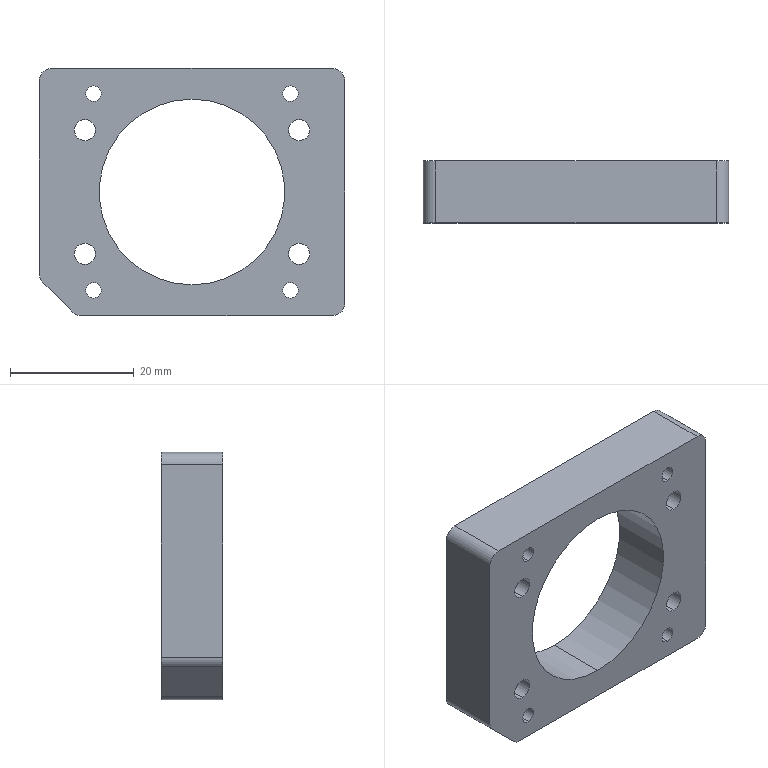Part | STEP file | 06-05KK60伺服连接Plate(KK60 Upper银伺服连接Plate) | 1 solid | 42 faces | box 49.4 x 10 x 40 mm | volume 11250 mm3 | cylinder 31 | plane 11 | commonest cylinder face diameters 2.5 x8 3.4 x8 6.5 x8 4 x5 30 x2
STEP:
#1=CARTESIAN_POINT('',(15.91,0.,14.66));
#2=VERTEX_POINT('',#1);
#3=CARTESIAN_POINT('',(15.91,0.,17.16));
#4=VERTEX_POINT('',#3);
#5=CARTESIAN_POINT('',(15.91,0.,15.91));
#6=DIRECTION('',(0.,1.,0.));
#7=DIRECTION('',(0.,0.,1.));
#8=AXIS2_PLACEMENT_3D('',#5,#6,#7);
#9=CIRCLE('',#8,1.25);
#10=EDGE_CURVE('',#2,#4,#9,.T.);
#11=ORIENTED_EDGE('',*,*,#10,.F.);
#12=CARTESIAN_POINT('',(15.91,10.,14.66));
#13=VERTEX_POINT('',#12);
#14=CARTESIAN_POINT('',(15.91,10.,14.66));
#15=DIRECTION('',(0.,1.,0.));
#16=VECTOR('',#15,1000.);
#17=LINE('',#14,#16);
#18=EDGE_CURVE('',#2,#13,#17,.T.);
#19=ORIENTED_EDGE('',*,*,#18,.T.);
#20=CARTESIAN_POINT('',(15.91,10.,17.16));
#21=VERTEX_POINT('',#20);
#22=CARTESIAN_POINT('',(15.91,10.,15.91));
#23=DIRECTION('',(0.,1.,0.));
#24=DIRECTION('',(0.,0.,1.));
#25=AXIS2_PLACEMENT_3D('',#22,#23,#24);
#26=CIRCLE('',#25,1.25);
#27=EDGE_CURVE('',#13,#21,#26,.T.);
#28=ORIENTED_EDGE('',*,*,#27,.T.);
#29=CARTESIAN_POINT('',(15.91,10.,17.16));
#30=DIRECTION('',(0.,1.,0.));
#31=VECTOR('',#30,1000.);
#32=LINE('',#29,#31);
#33=EDGE_CURVE('',#4,#21,#32,.T.);
#34=ORIENTED_EDGE('',*,*,#33,.F.);
#35=EDGE_LOOP('',(#11,#19,#28,#34));
#36=FACE_OUTER_BOUND('',#35,.T.);
#37=CARTESIAN_POINT('',(15.91,10.,15.91));
#38=DIRECTION('',(0.,1.,0.));
#39=DIRECTION('',(0.,0.,1.));
#40=AXIS2_PLACEMENT_3D('',#37,#38,#39);
#41=CYLINDRICAL_SURFACE('',#40,1.25);
#42=ADVANCED_FACE('',(#36),#41,.F.);
#43=CARTESIAN_POINT('',(-15.91,0.,14.66));
#44=VERTEX_POINT('',#43);
#45=CARTESIAN_POINT('',(-15.91,0.,17.16));
#46=VERTEX_POINT('',#45);
#47=CARTESIAN_POINT('',(-15.91,0.,15.91));
#48=DIRECTION('',(0.,1.,0.));
#49=DIRECTION('',(0.,0.,1.));
#50=AXIS2_PLACEMENT_3D('',#47,#48,#49);
#51=CIRCLE('',#50,1.25);
#52=EDGE_CURVE('',#44,#46,#51,.T.);
#53=ORIENTED_EDGE('',*,*,#52,.F.);
#54=CARTESIAN_POINT('',(-15.91,10.,14.66));
#55=VERTEX_POINT('',#54);
#56=CARTESIAN_POINT('',(-15.91,10.,14.66));
#57=DIRECTION('',(0.,1.,0.));
#58=VECTOR('',#57,1000.);
#59=LINE('',#56,#58);
#60=EDGE_CURVE('',#44,#55,#59,.T.);
#61=ORIENTED_EDGE('',*,*,#60,.T.);
#62=CARTESIAN_POINT('',(-15.91,10.,17.16));
#63=VERTEX_POINT('',#62);
#64=CARTESIAN_POINT('',(-15.91,10.,15.91));
#65=DIRECTION('',(0.,1.,0.));
#66=DIRECTION('',(0.,0.,1.));
#67=AXIS2_PLACEMENT_3D('',#64,#65,#66);
#68=CIRCLE('',#67,1.25);
#69=EDGE_CURVE('',#55,#63,#68,.T.);
#70=ORIENTED_EDGE('',*,*,#69,.T.);
#71=CARTESIAN_POINT('',(-15.91,10.,17.16));
#72=DIRECTION('',(0.,1.,0.));
#73=VECTOR('',#72,1000.);
#74=LINE('',#71,#73);
#75=EDGE_CURVE('',#46,#63,#74,.T.);
#76=ORIENTED_EDGE('',*,*,#75,.F.);
#77=EDGE_LOOP('',(#53,#61,#70,#76));
#78=FACE_OUTER_BOUND('',#77,.T.);
#79=CARTESIAN_POINT('',(-15.91,10.,15.91));
#80=DIRECTION('',(0.,1.,0.));
#81=DIRECTION('',(0.,0.,1.));
#82=AXIS2_PLACEMENT_3D('',#79,#80,#81);
#83=CYLINDRICAL_SURFACE('',#82,1.25);
#84=ADVANCED_FACE('',(#78),#83,.F.);
#85=CARTESIAN_POINT('',(-15.91,0.,-17.16));
#86=VERTEX_POINT('',#85);
#87=CARTESIAN_POINT('',(-15.91,0.,-14.66));
#88=VERTEX_POINT('',#87);
#89=CARTESIAN_POINT('',(-15.91,0.,-15.91));
#90=DIRECTION('',(0.,1.,0.));
#91=DIRECTION('',(0.,0.,1.));
#92=AXIS2_PLACEMENT_3D('',#89,#90,#91);
#93=CIRCLE('',#92,1.25);
#94=EDGE_CURVE('',#86,#88,#93,.T.);
#95=ORIENTED_EDGE('',*,*,#94,.F.);
#96=CARTESIAN_POINT('',(-15.91,10.,-17.16));
#97=VERTEX_POINT('',#96);
#98=CARTESIAN_POINT('',(-15.91,10.,-17.16));
#99=DIRECTION('',(0.,1.,0.));
#100=VECTOR('',#99,1000.);
#101=LINE('',#98,#100);
#102=EDGE_CURVE('',#86,#97,#101,.T.);
#103=ORIENTED_EDGE('',*,*,#102,.T.);
#104=CARTESIAN_POINT('',(-15.91,10.,-14.66));
#105=VERTEX_POINT('',#104);
#106=CARTESIAN_POINT('',(-15.91,10.,-15.91));
#107=DIRECTION('',(0.,1.,0.));
#108=DIRECTION('',(0.,0.,1.));
#109=AXIS2_PLACEMENT_3D('',#106,#107,#108);
#110=CIRCLE('',#109,1.25);
#111=EDGE_CURVE('',#97,#105,#110,.T.);
#112=ORIENTED_EDGE('',*,*,#111,.T.);
#113=CARTESIAN_POINT('',(-15.91,10.,-14.66));
#114=DIRECTION('',(0.,1.,0.));
#115=VECTOR('',#114,1000.);
#116=LINE('',#113,#115);
#117=EDGE_CURVE('',#88,#105,#116,.T.);
#118=ORIENTED_EDGE('',*,*,#117,.F.);
#119=EDGE_LOOP('',(#95,#103,#112,#118));
#120=FACE_OUTER_BOUND('',#119,.T.);
#121=CARTESIAN_POINT('',(-15.91,10.,-15.91));
#122=DIRECTION('',(0.,1.,0.));
#123=DIRECTION('',(0.,0.,1.));
#124=AXIS2_PLACEMENT_3D('',#121,#122,#123);
#125=CYLINDRICAL_SURFACE('',#124,1.25);
#126=ADVANCED_FACE('',(#120),#125,.F.);
#127=CARTESIAN_POINT('',(15.91,0.,-17.16));
#128=VERTEX_POINT('',#127);
#129=CARTESIAN_POINT('',(15.91,0.,-14.66));
#130=VERTEX_POINT('',#129);
#131=CARTESIAN_POINT('',(15.91,0.,-15.91));
#132=DIRECTION('',(0.,1.,0.));
#133=DIRECTION('',(0.,0.,1.));
#134=AXIS2_PLACEMENT_3D('',#131,#132,#133);
#135=CIRCLE('',#134,1.25);
#136=EDGE_CURVE('',#128,#130,#135,.T.);
#137=ORIENTED_EDGE('',*,*,#136,.F.);
#138=CARTESIAN_POINT('',(15.91,10.,-17.16));
#139=VERTEX_POINT('',#138);
#140=CARTESIAN_POINT('',(15.91,10.,-17.16));
#141=DIRECTION('',(0.,1.,0.));
#142=VECTOR('',#141,1000.);
#143=LINE('',#140,#142);
#144=EDGE_CURVE('',#128,#139,#143,.T.);
#145=ORIENTED_EDGE('',*,*,#144,.T.);
#146=CARTESIAN_POINT('',(15.91,10.,-14.66));
#147=VERTEX_POINT('',#146);
#148=CARTESIAN_POINT('',(15.91,10.,-15.91));
#149=DIRECTION('',(0.,1.,0.));
#150=DIRECTION('',(0.,0.,1.));
#151=AXIS2_PLACEMENT_3D('',#148,#149,#150);
#152=CIRCLE('',#151,1.25);
#153=EDGE_CURVE('',#139,#147,#152,.T.);
#154=ORIENTED_EDGE('',*,*,#153,.T.);
#155=CARTESIAN_POINT('',(15.91,10.,-14.66));
#156=DIRECTION('',(0.,1.,0.));
#157=VECTOR('',#156,1000.);
#158=LINE('',#155,#157);
#159=EDGE_CURVE('',#130,#147,#158,.T.);
#160=ORIENTED_EDGE('',*,*,#159,.F.);
#161=EDGE_LOOP('',(#137,#145,#154,#160));
#162=FACE_OUTER_BOUND('',#161,.T.);
#163=CARTESIAN_POINT('',(15.91,10.,-15.91));
#164=DIRECTION('',(0.,1.,0.));
#165=DIRECTION('',(0.,0.,1.));
#166=AXIS2_PLACEMENT_3D('',#163,#164,#165);
#167=CYLINDRICAL_SURFACE('',#166,1.25);
#168=ADVANCED_FACE('',(#162),#167,.F.);
#169=CARTESIAN_POINT('',(-17.321,3.,-13.25));
#170=VERTEX_POINT('',#169);
#171=CARTESIAN_POINT('',(-17.321,3.,-6.75));
#172=VERTEX_POINT('',#171);
#173=CARTESIAN_POINT('',(-17.321,3.,-10.));
#174=DIRECTION('',(0.,1.,0.));
#175=DIRECTION('',(0.,0.,1.));
#176=AXIS2_PLACEMENT_3D('',#173,#174,#175);
#177=CIRCLE('',#176,3.25);
#178=EDGE_CURVE('',#170,#172,#177,.T.);
#179=ORIENTED_EDGE('',*,*,#178,.F.);
#180=CARTESIAN_POINT('',(-17.321,10.,-13.25));
#181=VERTEX_POINT('',#180);
#182=CARTESIAN_POINT('',(-17.321,10.,-13.25));
#183=DIRECTION('',(0.,1.,0.));
#184=VECTOR('',#183,1000.);
#185=LINE('',#182,#184);
#186=EDGE_CURVE('',#170,#181,#185,.T.);
#187=ORIENTED_EDGE('',*,*,#186,.T.);
#188=CARTESIAN_POINT('',(-17.321,10.,-6.75));
#189=VERTEX_POINT('',#188);
#190=CARTESIAN_POINT('',(-17.321,10.,-10.));
#191=DIRECTION('',(0.,1.,0.));
#192=DIRECTION('',(0.,0.,1.));
#193=AXIS2_PLACEMENT_3D('',#190,#191,#192);
#194=CIRCLE('',#193,3.25);
#195=EDGE_CURVE('',#181,#189,#194,.T.);
#196=ORIENTED_EDGE('',*,*,#195,.T.);
#197=CARTESIAN_POINT('',(-17.321,10.,-6.75));
#198=DIRECTION('',(0.,1.,0.));
#199=VECTOR('',#198,1000.);
#200=LINE('',#197,#199);
#201=EDGE_CURVE('',#172,#189,#200,.T.);
#202=ORIENTED_EDGE('',*,*,#201,.F.);
#203=EDGE_LOOP('',(#179,#187,#196,#202));
#204=FACE_OUTER_BOUND('',#203,.T.);
#205=CARTESIAN_POINT('',(-17.321,10.,-10.));
#206=DIRECTION('',(0.,1.,0.));
#207=DIRECTION('',(0.,0.,1.));
#208=AXIS2_PLACEMENT_3D('',#205,#206,#207);
#209=CYLINDRICAL_SURFACE('',#208,3.25);
#210=ADVANCED_FACE('',(#204),#209,.F.);
#211=CARTESIAN_POINT('',(-17.321,0.,-11.7));
#212=VERTEX_POINT('',#211);
#213=CARTESIAN_POINT('',(-17.321,0.,-8.3));
#214=VERTEX_POINT('',#213);
#215=CARTESIAN_POINT('',(-17.321,0.,-10.));
#216=DIRECTION('',(0.,1.,0.));
#217=DIRECTION('',(0.,0.,1.));
#218=AXIS2_PLACEMENT_3D('',#215,#216,#217);
#219=CIRCLE('',#218,1.7);
#220=EDGE_CURVE('',#212,#214,#219,.T.);
#221=ORIENTED_EDGE('',*,*,#220,.F.);
#222=CARTESIAN_POINT('',(-17.321,3.,-11.7));
#223=VERTEX_POINT('',#222);
#224=CARTESIAN_POINT('',(-17.321,10.,-11.7));
#225=DIRECTION('',(0.,1.,0.));
#226=VECTOR('',#225,1000.);
#227=LINE('',#224,#226);
#228=EDGE_CURVE('',#212,#223,#227,.T.);
#229=ORIENTED_EDGE('',*,*,#228,.T.);
#230=CARTESIAN_POINT('',(-17.321,3.,-8.3));
#231=VERTEX_POINT('',#230);
#232=CARTESIAN_POINT('',(-17.321,3.,-10.));
#233=DIRECTION('',(0.,1.,0.));
#234=DIRECTION('',(0.,0.,1.));
#235=AXIS2_PLACEMENT_3D('',#232,#233,#234);
#236=CIRCLE('',#235,1.7);
#237=EDGE_CURVE('',#223,#231,#236,.T.);
#238=ORIENTED_EDGE('',*,*,#237,.T.);
#239=CARTESIAN_POINT('',(-17.321,10.,-8.3));
#240=DIRECTION('',(0.,1.,0.));
#241=VECTOR('',#240,1000.);
#242=LINE('',#239,#241);
#243=EDGE_CURVE('',#214,#231,#242,.T.);
#244=ORIENTED_EDGE('',*,*,#243,.F.);
#245=EDGE_LOOP('',(#221,#229,#238,#244));
#246=FACE_OUTER_BOUND('',#245,.T.);
#247=CARTESIAN_POINT('',(-17.321,10.,-10.));
#248=DIRECTION('',(0.,1.,0.));
#249=DIRECTION('',(0.,0.,1.));
#250=AXIS2_PLACEMENT_3D('',#247,#248,#249);
#251=CYLINDRICAL_SURFACE('',#250,1.7);
#252=ADVANCED_FACE('',(#246),#251,.F.);
#253=CARTESIAN_POINT('',(-17.321,3.,6.75));
#254=VERTEX_POINT('',#253);
#255=CARTESIAN_POINT('',(-17.321,3.,13.25));
#256=VERTEX_POINT('',#255);
#257=CARTESIAN_POINT('',(-17.321,3.,10.));
#258=DIRECTION('',(0.,1.,0.));
#259=DIRECTION('',(0.,0.,1.));
#260=AXIS2_PLACEMENT_3D('',#257,#258,#259);
#261=CIRCLE('',#260,3.25);
#262=EDGE_CURVE('',#254,#256,#261,.T.);
#263=ORIENTED_EDGE('',*,*,#262,.F.);
#264=CARTESIAN_POINT('',(-17.321,10.,6.75));
#265=VERTEX_POINT('',#264);
#266=CARTESIAN_POINT('',(-17.321,10.,6.75));
#267=DIRECTION('',(0.,1.,0.));
#268=VECTOR('',#267,1000.);
#269=LINE('',#266,#268);
#270=EDGE_CURVE('',#254,#265,#269,.T.);
#271=ORIENTED_EDGE('',*,*,#270,.T.);
#272=CARTESIAN_POINT('',(-17.321,10.,13.25));
#273=VERTEX_POINT('',#272);
#274=CARTESIAN_POINT('',(-17.321,10.,10.));
#275=DIRECTION('',(0.,1.,0.));
#276=DIRECTION('',(0.,0.,1.));
#277=AXIS2_PLACEMENT_3D('',#274,#275,#276);
#278=CIRCLE('',#277,3.25);
#279=EDGE_CURVE('',#265,#273,#278,.T.);
#280=ORIENTED_EDGE('',*,*,#279,.T.);
#281=CARTESIAN_POINT('',(-17.321,10.,13.25));
#282=DIRECTION('',(0.,1.,0.));
#283=VECTOR('',#282,1000.);
#284=LINE('',#281,#283);
#285=EDGE_CURVE('',#256,#273,#284,.T.);
#286=ORIENTED_EDGE('',*,*,#285,.F.);
#287=EDGE_LOOP('',(#263,#271,#280,#286));
#288=FACE_OUTER_BOUND('',#287,.T.);
#289=CARTESIAN_POINT('',(-17.321,10.,10.));
#290=DIRECTION('',(0.,1.,0.));
#291=DIRECTION('',(0.,0.,1.));
#292=AXIS2_PLACEMENT_3D('',#289,#290,#291);
#293=CYLINDRICAL_SURFACE('',#292,3.25);
#294=ADVANCED_FACE('',(#288),#293,.F.);
#295=CARTESIAN_POINT('',(-17.321,0.,8.3));
#296=VERTEX_POINT('',#295);
#297=CARTESIAN_POINT('',(-17.321,0.,11.7));
#298=VERTEX_POINT('',#297);
#299=CARTESIAN_POINT('',(-17.321,0.,10.));
#300=DIRECTION('',(0.,1.,0.));
#301=DIRECTION('',(0.,0.,1.));
#302=AXIS2_PLACEMENT_3D('',#299,#300,#301);
#303=CIRCLE('',#302,1.7);
#304=EDGE_CURVE('',#296,#298,#303,.T.);
#305=ORIENTED_EDGE('',*,*,#304,.F.);
#306=CARTESIAN_POINT('',(-17.321,3.,8.3));
#307=VERTEX_POINT('',#306);
#308=CARTESIAN_POINT('',(-17.321,10.,8.3));
#309=DIRECTION('',(0.,1.,0.));
#310=VECTOR('',#309,1000.);
#311=LINE('',#308,#310);
#312=EDGE_CURVE('',#296,#307,#311,.T.);
#313=ORIENTED_EDGE('',*,*,#312,.T.);
#314=CARTESIAN_POINT('',(-17.321,3.,11.7));
#315=VERTEX_POINT('',#314);
#316=CARTESIAN_POINT('',(-17.321,3.,10.));
#317=DIRECTION('',(0.,1.,0.));
#318=DIRECTION('',(0.,0.,1.));
#319=AXIS2_PLACEMENT_3D('',#316,#317,#318);
#320=CIRCLE('',#319,1.7);
#321=EDGE_CURVE('',#307,#315,#320,.T.);
#322=ORIENTED_EDGE('',*,*,#321,.T.);
#323=CARTESIAN_POINT('',(-17.321,10.,11.7));
#324=DIRECTION('',(0.,1.,0.));
#325=VECTOR('',#324,1000.);
#326=LINE('',#323,#325);
#327=EDGE_CURVE('',#298,#315,#326,.T.);
#328=ORIENTED_EDGE('',*,*,#327,.F.);
#329=EDGE_LOOP('',(#305,#313,#322,#328));
#330=FACE_OUTER_BOUND('',#329,.T.);
#331=CARTESIAN_POINT('',(-17.321,10.,10.));
#332=DIRECTION('',(0.,1.,0.));
#333=DIRECTION('',(0.,0.,1.));
#334=AXIS2_PLACEMENT_3D('',#331,#332,#333);
#335=CYLINDRICAL_SURFACE('',#334,1.7);
#336=ADVANCED_FACE('',(#330),#335,.F.);
#337=CARTESIAN_POINT('',(17.321,3.,6.75));
#338=VERTEX_POINT('',#337);
#339=CARTESIAN_POINT('',(17.321,3.,13.25));
#340=VERTEX_POINT('',#339);
#341=CARTESIAN_POINT('',(17.321,3.,10.));
#342=DIRECTION('',(0.,1.,0.));
#343=DIRECTION('',(0.,0.,1.));
#344=AXIS2_PLACEMENT_3D('',#341,#342,#343);
#345=CIRCLE('',#344,3.25);
#346=EDGE_CURVE('',#338,#340,#345,.T.);
#347=ORIENTED_EDGE('',*,*,#346,.F.);
#348=CARTESIAN_POINT('',(17.321,10.,6.75));
#349=VERTEX_POINT('',#348);
#350=CARTESIAN_POINT('',(17.321,10.,6.75));
#351=DIRECTION('',(0.,1.,0.));
#352=VECTOR('',#351,1000.);
#353=LINE('',#350,#352);
#354=EDGE_CURVE('',#338,#349,#353,.T.);
#355=ORIENTED_EDGE('',*,*,#354,.T.);
#356=CARTESIAN_POINT('',(17.321,10.,13.25));
#357=VERTEX_POINT('',#356);
#358=CARTESIAN_POINT('',(17.321,10.,10.));
#359=DIRECTION('',(0.,1.,0.));
#360=DIRECTION('',(0.,0.,1.));
#361=AXIS2_PLACEMENT_3D('',#358,#359,#360);
#362=CIRCLE('',#361,3.25);
#363=EDGE_CURVE('',#349,#357,#362,.T.);
#364=ORIENTED_EDGE('',*,*,#363,.T.);
#365=CARTESIAN_POINT('',(17.321,10.,13.25));
#366=DIRECTION('',(0.,1.,0.));
#367=VECTOR('',#366,1000.);
#368=LINE('',#365,#367);
#369=EDGE_CURVE('',#340,#357,#368,.T.);
#370=ORIENTED_EDGE('',*,*,#369,.F.);
#371=EDGE_LOOP('',(#347,#355,#364,#370));
#372=FACE_OUTER_BOUND('',#371,.T.);
#373=CARTESIAN_POINT('',(17.321,10.,10.));
#374=DIRECTION('',(0.,1.,0.));
#375=DIRECTION('',(0.,0.,1.));
#376=AXIS2_PLACEMENT_3D('',#373,#374,#375);
#377=CYLINDRICAL_SURFACE('',#376,3.25);
#378=ADVANCED_FACE('',(#372),#377,.F.);
#379=CARTESIAN_POINT('',(17.321,0.,8.3));
#380=VERTEX_POINT('',#379);
#381=CARTESIAN_POINT('',(17.321,0.,11.7));
#382=VERTEX_POINT('',#381);
#383=CARTESIAN_POINT('',(17.321,0.,10.));
#384=DIRECTION('',(0.,1.,0.));
#385=DIRECTION('',(0.,0.,1.));
#386=AXIS2_PLACEMENT_3D('',#383,#384,#385);
#387=CIRCLE('',#386,1.7);
#388=EDGE_CURVE('',#380,#382,#387,.T.);
#389=ORIENTED_EDGE('',*,*,#388,.F.);
#390=CARTESIAN_POINT('',(17.321,3.,8.3));
#391=VERTEX_POINT('',#390);
#392=CARTESIAN_POINT('',(17.321,10.,8.3));
#393=DIRECTION('',(0.,1.,0.));
#394=VECTOR('',#393,1000.);
#395=LINE('',#392,#394);
#396=EDGE_CURVE('',#380,#391,#395,.T.);
#397=ORIENTED_EDGE('',*,*,#396,.T.);
#398=CARTESIAN_POINT('',(17.321,3.,11.7));
#399=VERTEX_POINT('',#398);
#400=CARTESIAN_POINT('',(17.321,3.,10.));
#401=DIRECTION('',(0.,1.,0.));
#402=DIRECTION('',(0.,0.,1.));
#403=AXIS2_PLACEMENT_3D('',#400,#401,#402);
#404=CIRCLE('',#403,1.7);
#405=EDGE_CURVE('',#391,#399,#404,.T.);
#406=ORIENTED_EDGE('',*,*,#405,.T.);
#407=CARTESIAN_POINT('',(17.321,10.,11.7));
#408=DIRECTION('',(0.,1.,0.));
#409=VECTOR('',#408,1000.);
#410=LINE('',#407,#409);
#411=EDGE_CURVE('',#382,#399,#410,.T.);
#412=ORIENTED_EDGE('',*,*,#411,.F.);
#413=EDGE_LOOP('',(#389,#397,#406,#412));
#414=FACE_OUTER_BOUND('',#413,.T.);
#415=CARTESIAN_POINT('',(17.321,10.,10.));
#416=DIRECTION('',(0.,1.,0.));
#417=DIRECTION('',(0.,0.,1.));
#418=AXIS2_PLACEMENT_3D('',#415,#416,#417);
#419=CYLINDRICAL_SURFACE('',#418,1.7);
#420=ADVANCED_FACE('',(#414),#419,.F.);
#421=CARTESIAN_POINT('',(17.321,3.,-13.25));
#422=VERTEX_POINT('',#421);
#423=CARTESIAN_POINT('',(17.321,3.,-6.75));
#424=VERTEX_POINT('',#423);
#425=CARTESIAN_POINT('',(17.321,3.,-10.));
#426=DIRECTION('',(0.,1.,0.));
#427=DIRECTION('',(0.,0.,1.));
#428=AXIS2_PLACEMENT_3D('',#425,#426,#427);
#429=CIRCLE('',#428,3.25);
#430=EDGE_CURVE('',#422,#424,#429,.T.);
#431=ORIENTED_EDGE('',*,*,#430,.F.);
#432=CARTESIAN_POINT('',(17.321,10.,-13.25));
#433=VERTEX_POINT('',#432);
#434=CARTESIAN_POINT('',(17.321,10.,-13.25));
#435=DIRECTION('',(0.,1.,0.));
#436=VECTOR('',#435,1000.);
#437=LINE('',#434,#436);
#438=EDGE_CURVE('',#422,#433,#437,.T.);
#439=ORIENTED_EDGE('',*,*,#438,.T.);
#440=CARTESIAN_POINT('',(17.321,10.,-6.75));
#441=VERTEX_POINT('',#440);
#442=CARTESIAN_POINT('',(17.321,10.,-10.));
#443=DIRECTION('',(0.,1.,0.));
#444=DIRECTION('',(0.,0.,1.));
#445=AXIS2_PLACEMENT_3D('',#442,#443,#444);
#446=CIRCLE('',#445,3.25);
#447=EDGE_CURVE('',#433,#441,#446,.T.);
#448=ORIENTED_EDGE('',*,*,#447,.T.);
#449=CARTESIAN_POINT('',(17.321,10.,-6.75));
#450=DIRECTION('',(0.,1.,0.));
#451=VECTOR('',#450,1000.);
#452=LINE('',#449,#451);
#453=EDGE_CURVE('',#424,#441,#452,.T.);
#454=ORIENTED_EDGE('',*,*,#453,.F.);
#455=EDGE_LOOP('',(#431,#439,#448,#454));
#456=FACE_OUTER_BOUND('',#455,.T.);
#457=CARTESIAN_POINT('',(17.321,10.,-10.));
#458=DIRECTION('',(0.,1.,0.));
#459=DIRECTION('',(0.,0.,1.));
#460=AXIS2_PLACEMENT_3D('',#457,#458,#459);
#461=CYLINDRICAL_SURFACE('',#460,3.25);
#462=ADVANCED_FACE('',(#456),#461,.F.);
#463=CARTESIAN_POINT('',(17.321,0.,-11.7));
#464=VERTEX_POINT('',#463);
#465=CARTESIAN_POINT('',(17.321,0.,-8.3));
#466=VERTEX_POINT('',#465);
#467=CARTESIAN_POINT('',(17.321,0.,-10.));
#468=DIRECTION('',(0.,1.,0.));
#469=DIRECTION('',(0.,0.,1.));
#470=AXIS2_PLACEMENT_3D('',#467,#468,#469);
#471=CIRCLE('',#470,1.7);
#472=EDGE_CURVE('',#464,#466,#471,.T.);
#473=ORIENTED_EDGE('',*,*,#472,.F.);
#474=CARTESIAN_POINT('',(17.321,3.,-11.7));
#475=VERTEX_POINT('',#474);
#476=CARTESIAN_POINT('',(17.321,10.,-11.7));
#477=DIRECTION('',(0.,1.,0.));
#478=VECTOR('',#477,1000.);
#479=LINE('',#476,#478);
#480=EDGE_CURVE('',#464,#475,#479,.T.);
#481=ORIENTED_EDGE('',*,*,#480,.T.);
#482=CARTESIAN_POINT('',(17.321,3.,-8.3));
#483=VERTEX_POINT('',#482);
#484=CARTESIAN_POINT('',(17.321,3.,-10.));
#485=DIRECTION('',(0.,1.,0.));
#486=DIRECTION('',(0.,0.,1.));
#487=AXIS2_PLACEMENT_3D('',#484,#485,#486);
#488=CIRCLE('',#487,1.7);
#489=EDGE_CURVE('',#475,#483,#488,.T.);
#490=ORIENTED_EDGE('',*,*,#489,.T.);
#491=CARTESIAN_POINT('',(17.321,10.,-8.3));
#492=DIRECTION('',(0.,1.,0.));
#493=VECTOR('',#492,1000.);
#494=LINE('',#491,#493);
#495=EDGE_CURVE('',#466,#483,#494,.T.);
#496=ORIENTED_EDGE('',*,*,#495,.F.);
#497=EDGE_LOOP('',(#473,#481,#490,#496));
#498=FACE_OUTER_BOUND('',#497,.T.);
#499=CARTESIAN_POINT('',(17.321,10.,-10.));
#500=DIRECTION('',(0.,1.,0.));
#501=DIRECTION('',(0.,0.,1.));
#502=AXIS2_PLACEMENT_3D('',#499,#500,#501);
#503=CYLINDRICAL_SURFACE('',#502,1.7);
#504=ADVANCED_FACE('',(#498),#503,.F.);
#505=CARTESIAN_POINT('',(0.,0.,-15.));
#506=VERTEX_POINT('',#505);
#507=CARTESIAN_POINT('',(0.,0.,15.));
#508=VERTEX_POINT('',#507);
#509=CARTESIAN_POINT('',(0.,0.,0.));
#510=DIRECTION('',(0.,1.,0.));
#511=DIRECTION('',(0.,0.,1.));
#512=AXIS2_PLACEMENT_3D('',#509,#510,#511);
#513=CIRCLE('',#512,15.);
#514=EDGE_CURVE('',#506,#508,#513,.T.);
#515=ORIENTED_EDGE('',*,*,#514,.F.);
#516=CARTESIAN_POINT('',(0.,10.,-15.));
#517=VERTEX_POINT('',#516);
#518=CARTESIAN_POINT('',(0.,0.,-15.));
#519=DIRECTION('',(0.,1.,0.));
#520=VECTOR('',#519,1000.);
#521=LINE('',#518,#520);
#522=EDGE_CURVE('',#506,#517,#521,.T.);
#523=ORIENTED_EDGE('',*,*,#522,.T.);
#524=CARTESIAN_POINT('',(0.,10.,15.));
#525=VERTEX_POINT('',#524);
#526=CARTESIAN_POINT('',(0.,10.,0.));
#527=DIRECTION('',(0.,1.,0.));
#528=DIRECTION('',(0.,0.,1.));
#529=AXIS2_PLACEMENT_3D('',#526,#527,#528);
#530=CIRCLE('',#529,15.);
#531=EDGE_CURVE('',#517,#525,#530,.T.);
#532=ORIENTED_EDGE('',*,*,#531,.T.);
#533=CARTESIAN_POINT('',(0.,0.,15.));
#534=DIRECTION('',(0.,1.,0.));
#535=VECTOR('',#534,1000.);
#536=LINE('',#533,#535);
#537=EDGE_CURVE('',#508,#525,#536,.T.);
#538=ORIENTED_EDGE('',*,*,#537,.F.);
#539=EDGE_LOOP('',(#515,#523,#532,#538));
#540=FACE_OUTER_BOUND('',#539,.T.);
#541=CARTESIAN_POINT('',(0.,0.,0.));
#542=DIRECTION('',(0.,1.,0.));
#543=DIRECTION('',(0.,0.,1.));
#544=AXIS2_PLACEMENT_3D('',#541,#542,#543);
#545=CYLINDRICAL_SURFACE('',#544,15.);
#546=ADVANCED_FACE('',(#540),#545,.F.);
#547=CARTESIAN_POINT('',(24.7,10.,18.));
#548=VERTEX_POINT('',#547);
#549=CARTESIAN_POINT('',(24.7,10.,-18.));
#550=VERTEX_POINT('',#549);
#551=CARTESIAN_POINT('',(24.7,10.,20.));
#552=DIRECTION('',(0.,0.,-1.));
#553=VECTOR('',#552,1000.);
#554=LINE('',#551,#553);
#555=EDGE_CURVE('',#548,#550,#554,.T.);
#556=ORIENTED_EDGE('',*,*,#555,.F.);
#557=CARTESIAN_POINT('',(24.7,0.,18.));
#558=VERTEX_POINT('',#557);
#559=CARTESIAN_POINT('',(24.7,10.,18.));
#560=DIRECTION('',(0.,-1.,0.));
#561=VECTOR('',#560,1000.);
#562=LINE('',#559,#561);
#563=EDGE_CURVE('',#548,#558,#562,.T.);
#564=ORIENTED_EDGE('',*,*,#563,.T.);
#565=CARTESIAN_POINT('',(24.7,0.,-18.));
#566=VERTEX_POINT('',#565);
#567=CARTESIAN_POINT('',(24.7,0.,20.));
#568=DIRECTION('',(0.,0.,-1.));
#569=VECTOR('',#568,1000.);
#570=LINE('',#567,#569);
#571=EDGE_CURVE('',#558,#566,#570,.T.);
#572=ORIENTED_EDGE('',*,*,#571,.T.);
#573=CARTESIAN_POINT('',(24.7,10.,-18.));
#574=DIRECTION('',(0.,1.,0.));
#575=VECTOR('',#574,1000.);
#576=LINE('',#573,#575);
#577=EDGE_CURVE('',#566,#550,#576,.T.);
#578=ORIENTED_EDGE('',*,*,#577,.T.);
#579=EDGE_LOOP('',(#556,#564,#572,#578));
#580=FACE_OUTER_BOUND('',#579,.T.);
#581=CARTESIAN_POINT('',(24.7,10.,20.));
#582=DIRECTION('',(-1.,0.,0.));
#583=DIRECTION('',(0.,0.,1.));
#584=AXIS2_PLACEMENT_3D('',#581,#582,#583);
#585=PLANE('',#584);
#586=ADVANCED_FACE('',(#580),#585,.F.);
#587=CARTESIAN_POINT('',(22.7,10.,-20.));
#588=VERTEX_POINT('',#587);
#589=CARTESIAN_POINT('',(-17.872,10.,-20.));
#590=VERTEX_POINT('',#589);
#591=CARTESIAN_POINT('',(-24.7,10.,-20.));
#592=DIRECTION('',(-1.,0.,0.));
#593=VECTOR('',#592,1000.);
#594=LINE('',#591,#593);
#595=EDGE_CURVE('',#588,#590,#594,.T.);
#596=ORIENTED_EDGE('',*,*,#595,.F.);
#597=CARTESIAN_POINT('',(22.7,0.,-20.));
#598=VERTEX_POINT('',#597);
#599=CARTESIAN_POINT('',(22.7,10.,-20.));
#600=DIRECTION('',(0.,-1.,0.));
#601=VECTOR('',#600,1000.);
#602=LINE('',#599,#601);
#603=EDGE_CURVE('',#588,#598,#602,.T.);
#604=ORIENTED_EDGE('',*,*,#603,.T.);
#605=CARTESIAN_POINT('',(-17.872,0.,-20.));
#606=VERTEX_POINT('',#605);
#607=CARTESIAN_POINT('',(-24.7,0.,-20.));
#608=DIRECTION('',(-1.,0.,0.));
#609=VECTOR('',#608,1000.);
#610=LINE('',#607,#609);
#611=EDGE_CURVE('',#598,#606,#610,.T.);
#612=ORIENTED_EDGE('',*,*,#611,.T.);
#613=CARTESIAN_POINT('',(-17.872,10.,-20.));
#614=DIRECTION('',(0.,1.,0.));
#615=VECTOR('',#614,1000.);
#616=LINE('',#613,#615);
#617=EDGE_CURVE('',#606,#590,#616,.T.);
#618=ORIENTED_EDGE('',*,*,#617,.T.);
#619=EDGE_LOOP('',(#596,#604,#612,#618));
#620=FACE_OUTER_BOUND('',#619,.T.);
#621=CARTESIAN_POINT('',(-24.7,10.,-20.));
#622=DIRECTION('',(0.,0.,1.));
#623=DIRECTION('',(1.,0.,0.));
#624=AXIS2_PLACEMENT_3D('',#621,#622,#623);
#625=PLANE('',#624);
#626=ADVANCED_FACE('',(#620),#625,.F.);
#627=CARTESIAN_POINT('',(-24.7,0.,-13.172));
#628=VERTEX_POINT('',#627);
#629=CARTESIAN_POINT('',(-24.7,0.,18.));
#630=VERTEX_POINT('',#629);
#631=CARTESIAN_POINT('',(-24.7,0.,20.));
#632=DIRECTION('',(0.,0.,1.));
#633=VECTOR('',#632,1000.);
#634=LINE('',#631,#633);
#635=EDGE_CURVE('',#628,#630,#634,.T.);
#636=ORIENTED_EDGE('',*,*,#635,.T.);
#637=CARTESIAN_POINT('',(-24.7,10.,18.));
#638=VERTEX_POINT('',#637);
#639=CARTESIAN_POINT('',(-24.7,10.,18.));
#640=DIRECTION('',(0.,1.,0.));
#641=VECTOR('',#640,1000.);
#642=LINE('',#639,#641);
#643=EDGE_CURVE('',#630,#638,#642,.T.);
#644=ORIENTED_EDGE('',*,*,#643,.T.);
#645=CARTESIAN_POINT('',(-24.7,10.,-13.172));
#646=VERTEX_POINT('',#645);
#647=CARTESIAN_POINT('',(-24.7,10.,20.));
#648=DIRECTION('',(0.,0.,1.));
#649=VECTOR('',#648,1000.);
#650=LINE('',#647,#649);
#651=EDGE_CURVE('',#646,#638,#650,.T.);
#652=ORIENTED_EDGE('',*,*,#651,.F.);
#653=CARTESIAN_POINT('',(-24.7,0.,-13.172));
#654=DIRECTION('',(0.,-1.,0.));
#655=VECTOR('',#654,1000.);
#656=LINE('',#653,#655);
#657=EDGE_CURVE('',#646,#628,#656,.T.);
#658=ORIENTED_EDGE('',*,*,#657,.T.);
#659=EDGE_LOOP('',(#636,#644,#652,#658));
#660=FACE_OUTER_BOUND('',#659,.T.);
#661=CARTESIAN_POINT('',(-24.7,10.,20.));
#662=DIRECTION('',(1.,0.,0.));
#663=DIRECTION('',(0.,0.,-1.));
#664=AXIS2_PLACEMENT_3D('',#661,#662,#663);
#665=PLANE('',#664);
#666=ADVANCED_FACE('',(#660),#665,.F.);
#667=CARTESIAN_POINT('',(-22.7,10.,20.));
#668=VERTEX_POINT('',#667);
#669=CARTESIAN_POINT('',(22.7,10.,20.));
#670=VERTEX_POINT('',#669);
#671=CARTESIAN_POINT('',(-24.7,10.,20.));
#672=DIRECTION('',(1.,0.,0.));
#673=VECTOR('',#672,1000.);
#674=LINE('',#671,#673);
#675=EDGE_CURVE('',#668,#670,#674,.T.);
#676=ORIENTED_EDGE('',*,*,#675,.F.);
#677=CARTESIAN_POINT('',(-22.7,0.,20.));
#678=VERTEX_POINT('',#677);
#679=CARTESIAN_POINT('',(-22.7,10.,20.));
#680=DIRECTION('',(0.,-1.,0.));
#681=VECTOR('',#680,1000.);
#682=LINE('',#679,#681);
#683=EDGE_CURVE('',#668,#678,#682,.T.);
#684=ORIENTED_EDGE('',*,*,#683,.T.);
#685=CARTESIAN_POINT('',(22.7,0.,20.));
#686=VERTEX_POINT('',#685);
#687=CARTESIAN_POINT('',(-24.7,0.,20.));
#688=DIRECTION('',(1.,0.,0.));
#689=VECTOR('',#688,1000.);
#690=LINE('',#687,#689);
#691=EDGE_CURVE('',#678,#686,#690,.T.);
#692=ORIENTED_EDGE('',*,*,#691,.T.);
#693=CARTESIAN_POINT('',(22.7,10.,20.));
#694=DIRECTION('',(0.,1.,0.));
#695=VECTOR('',#694,1000.);
#696=LINE('',#693,#695);
#697=EDGE_CURVE('',#686,#670,#696,.T.);
#698=ORIENTED_EDGE('',*,*,#697,.T.);
#699=EDGE_LOOP('',(#676,#684,#692,#698));
#700=FACE_OUTER_BOUND('',#699,.T.);
#701=CARTESIAN_POINT('',(-24.7,10.,20.));
#702=DIRECTION('',(0.,0.,-1.));
#703=DIRECTION('',(-1.,0.,0.));
#704=AXIS2_PLACEMENT_3D('',#701,#702,#703);
#705=PLANE('',#704);
#706=ADVANCED_FACE('',(#700),#705,.F.);
#707=CARTESIAN_POINT('',(15.91,10.,15.91));
#708=DIRECTION('',(0.,1.,0.));
#709=DIRECTION('',(0.,0.,1.));
#710=AXIS2_PLACEMENT_3D('',#707,#708,#709);
#711=CIRCLE('',#710,1.25);
#712=EDGE_CURVE('',#21,#13,#711,.T.);
#713=ORIENTED_EDGE('',*,*,#712,.F.);
#714=ORIENTED_EDGE('',*,*,#27,.F.);
#715=EDGE_LOOP('',(#713,#714));
#716=FACE_BOUND('',#715,.T.);
#717=CARTESIAN_POINT('',(-15.91,10.,15.91));
#718=DIRECTION('',(0.,1.,0.));
#719=DIRECTION('',(0.,0.,1.));
#720=AXIS2_PLACEMENT_3D('',#717,#718,#719);
#721=CIRCLE('',#720,1.25);
#722=EDGE_CURVE('',#63,#55,#721,.T.);
#723=ORIENTED_EDGE('',*,*,#722,.F.);
#724=ORIENTED_EDGE('',*,*,#69,.F.);
#725=EDGE_LOOP('',(#723,#724));
#726=FACE_BOUND('',#725,.T.);
#727=CARTESIAN_POINT('',(-15.91,10.,-15.91));
#728=DIRECTION('',(0.,1.,0.));
#729=DIRECTION('',(0.,0.,1.));
#730=AXIS2_PLACEMENT_3D('',#727,#728,#729);
#731=CIRCLE('',#730,1.25);
#732=EDGE_CURVE('',#105,#97,#731,.T.);
#733=ORIENTED_EDGE('',*,*,#732,.F.);
#734=ORIENTED_EDGE('',*,*,#111,.F.);
#735=EDGE_LOOP('',(#733,#734));
#736=FACE_BOUND('',#735,.T.);
#737=CARTESIAN_POINT('',(15.91,10.,-15.91));
#738=DIRECTION('',(0.,1.,0.));
#739=DIRECTION('',(0.,0.,1.));
#740=AXIS2_PLACEMENT_3D('',#737,#738,#739);
#741=CIRCLE('',#740,1.25);
#742=EDGE_CURVE('',#147,#139,#741,.T.);
#743=ORIENTED_EDGE('',*,*,#742,.F.);
#744=ORIENTED_EDGE('',*,*,#153,.F.);
#745=EDGE_LOOP('',(#743,#744));
#746=FACE_BOUND('',#745,.T.);
#747=CARTESIAN_POINT('',(-17.321,10.,-10.));
#748=DIRECTION('',(0.,1.,0.));
#749=DIRECTION('',(0.,0.,1.));
#750=AXIS2_PLACEMENT_3D('',#747,#748,#749);
#751=CIRCLE('',#750,3.25);
#752=EDGE_CURVE('',#189,#181,#751,.T.);
#753=ORIENTED_EDGE('',*,*,#752,.F.);
#754=ORIENTED_EDGE('',*,*,#195,.F.);
#755=EDGE_LOOP('',(#753,#754));
#756=FACE_BOUND('',#755,.T.);
#757=CARTESIAN_POINT('',(-17.321,10.,10.));
#758=DIRECTION('',(0.,1.,0.));
#759=DIRECTION('',(0.,0.,1.));
#760=AXIS2_PLACEMENT_3D('',#757,#758,#759);
#761=CIRCLE('',#760,3.25);
#762=EDGE_CURVE('',#273,#265,#761,.T.);
#763=ORIENTED_EDGE('',*,*,#762,.F.);
#764=ORIENTED_EDGE('',*,*,#279,.F.);
#765=EDGE_LOOP('',(#763,#764));
#766=FACE_BOUND('',#765,.T.);
#767=CARTESIAN_POINT('',(17.321,10.,10.));
#768=DIRECTION('',(0.,1.,0.));
#769=DIRECTION('',(0.,0.,1.));
#770=AXIS2_PLACEMENT_3D('',#767,#768,#769);
#771=CIRCLE('',#770,3.25);
#772=EDGE_CURVE('',#357,#349,#771,.T.);
#773=ORIENTED_EDGE('',*,*,#772,.F.);
#774=ORIENTED_EDGE('',*,*,#363,.F.);
#775=EDGE_LOOP('',(#773,#774));
#776=FACE_BOUND('',#775,.T.);
#777=CARTESIAN_POINT('',(17.321,10.,-10.));
#778=DIRECTION('',(0.,1.,0.));
#779=DIRECTION('',(0.,0.,1.));
#780=AXIS2_PLACEMENT_3D('',#777,#778,#779);
#781=CIRCLE('',#780,3.25);
#782=EDGE_CURVE('',#441,#433,#781,.T.);
#783=ORIENTED_EDGE('',*,*,#782,.F.);
#784=ORIENTED_EDGE('',*,*,#447,.F.);
#785=EDGE_LOOP('',(#783,#784));
#786=FACE_BOUND('',#785,.T.);
#787=CARTESIAN_POINT('',(0.,10.,0.));
#788=DIRECTION('',(0.,1.,0.));
#789=DIRECTION('',(0.,0.,1.));
#790=AXIS2_PLACEMENT_3D('',#787,#788,#789);
#791=CIRCLE('',#790,15.);
#792=EDGE_CURVE('',#525,#517,#791,.T.);
#793=ORIENTED_EDGE('',*,*,#792,.F.);
#794=ORIENTED_EDGE('',*,*,#531,.F.);
#795=EDGE_LOOP('',(#793,#794));
#796=FACE_BOUND('',#795,.T.);
#797=ORIENTED_EDGE('',*,*,#651,.T.);
#798=CARTESIAN_POINT('',(-22.7,10.,18.));
#799=DIRECTION('',(0.,1.,0.));
#800=DIRECTION('',(0.,0.,-1.));
#801=AXIS2_PLACEMENT_3D('',#798,#799,#800);
#802=CIRCLE('',#801,2.);
#803=EDGE_CURVE('',#638,#668,#802,.T.);
#804=ORIENTED_EDGE('',*,*,#803,.T.);
#805=ORIENTED_EDGE('',*,*,#675,.T.);
#806=CARTESIAN_POINT('',(22.7,10.,18.));
#807=DIRECTION('',(0.,1.,0.));
#808=DIRECTION('',(0.,0.,-1.));
#809=AXIS2_PLACEMENT_3D('',#806,#807,#808);
#810=CIRCLE('',#809,2.);
#811=EDGE_CURVE('',#670,#548,#810,.T.);
#812=ORIENTED_EDGE('',*,*,#811,.T.);
#813=ORIENTED_EDGE('',*,*,#555,.T.);
#814=CARTESIAN_POINT('',(22.7,10.,-18.));
#815=DIRECTION('',(0.,1.,0.));
#816=DIRECTION('',(0.,0.,-1.));
#817=AXIS2_PLACEMENT_3D('',#814,#815,#816);
#818=CIRCLE('',#817,2.);
#819=EDGE_CURVE('',#550,#588,#818,.T.);
#820=ORIENTED_EDGE('',*,*,#819,.T.);
#821=ORIENTED_EDGE('',*,*,#595,.T.);
#822=CARTESIAN_POINT('',(-19.286,10.,-19.414));
#823=VERTEX_POINT('',#822);
#824=CARTESIAN_POINT('',(-17.872,10.,-18.));
#825=DIRECTION('',(0.,1.,0.));
#826=DIRECTION('',(0.,0.,-1.));
#827=AXIS2_PLACEMENT_3D('',#824,#825,#826);
#828=CIRCLE('',#827,2.);
#829=EDGE_CURVE('',#590,#823,#828,.T.);
#830=ORIENTED_EDGE('',*,*,#829,.T.);
#831=CARTESIAN_POINT('',(-24.114,10.,-14.586));
#832=VERTEX_POINT('',#831);
#833=CARTESIAN_POINT('',(-24.7,10.,-14.));
#834=DIRECTION('',(-0.7071,0.,0.7071));
#835=VECTOR('',#834,1000.);
#836=LINE('',#833,#835);
#837=EDGE_CURVE('',#823,#832,#836,.T.);
#838=ORIENTED_EDGE('',*,*,#837,.T.);
#839=CARTESIAN_POINT('',(-22.7,10.,-13.172));
#840=DIRECTION('',(0.,1.,0.));
#841=DIRECTION('',(0.,0.,-1.));
#842=AXIS2_PLACEMENT_3D('',#839,#840,#841);
#843=CIRCLE('',#842,2.);
#844=EDGE_CURVE('',#832,#646,#843,.T.);
#845=ORIENTED_EDGE('',*,*,#844,.T.);
#846=EDGE_LOOP('',(#797,#804,#805,#812,#813,#820,#821,#830,#838,#845));
#847=FACE_OUTER_BOUND('',#846,.T.);
#848=CARTESIAN_POINT('',(24.7,10.,-20.));
#849=DIRECTION('',(0.,-1.,0.));
#850=DIRECTION('',(0.,0.,-1.));
#851=AXIS2_PLACEMENT_3D('',#848,#849,#850);
#852=PLANE('',#851);
#853=ADVANCED_FACE('',(#716,#726,#736,#746,#756,#766,#776,#786,#796,#847),#852,.F.);
#854=CARTESIAN_POINT('',(15.91,0.,15.91));
#855=DIRECTION('',(0.,1.,0.));
#856=DIRECTION('',(0.,0.,1.));
#857=AXIS2_PLACEMENT_3D('',#854,#855,#856);
#858=CIRCLE('',#857,1.25);
#859=EDGE_CURVE('',#4,#2,#858,.T.);
#860=ORIENTED_EDGE('',*,*,#859,.T.);
#861=ORIENTED_EDGE('',*,*,#10,.T.);
#862=EDGE_LOOP('',(#860,#861));
#863=FACE_BOUND('',#862,.T.);
#864=CARTESIAN_POINT('',(-15.91,0.,15.91));
#865=DIRECTION('',(0.,1.,0.));
#866=DIRECTION('',(0.,0.,1.));
#867=AXIS2_PLACEMENT_3D('',#864,#865,#866);
#868=CIRCLE('',#867,1.25);
#869=EDGE_CURVE('',#46,#44,#868,.T.);
#870=ORIENTED_EDGE('',*,*,#869,.T.);
#871=ORIENTED_EDGE('',*,*,#52,.T.);
#872=EDGE_LOOP('',(#870,#871));
#873=FACE_BOUND('',#872,.T.);
#874=CARTESIAN_POINT('',(-15.91,0.,-15.91));
#875=DIRECTION('',(0.,1.,0.));
#876=DIRECTION('',(0.,0.,1.));
#877=AXIS2_PLACEMENT_3D('',#874,#875,#876);
#878=CIRCLE('',#877,1.25);
#879=EDGE_CURVE('',#88,#86,#878,.T.);
#880=ORIENTED_EDGE('',*,*,#879,.T.);
#881=ORIENTED_EDGE('',*,*,#94,.T.);
#882=EDGE_LOOP('',(#880,#881));
#883=FACE_BOUND('',#882,.T.);
#884=CARTESIAN_POINT('',(15.91,0.,-15.91));
#885=DIRECTION('',(0.,1.,0.));
#886=DIRECTION('',(0.,0.,1.));
#887=AXIS2_PLACEMENT_3D('',#884,#885,#886);
#888=CIRCLE('',#887,1.25);
#889=EDGE_CURVE('',#130,#128,#888,.T.);
#890=ORIENTED_EDGE('',*,*,#889,.T.);
#891=ORIENTED_EDGE('',*,*,#136,.T.);
#892=EDGE_LOOP('',(#890,#891));
#893=FACE_BOUND('',#892,.T.);
#894=CARTESIAN_POINT('',(-17.321,0.,-10.));
#895=DIRECTION('',(0.,1.,0.));
#896=DIRECTION('',(0.,0.,1.));
#897=AXIS2_PLACEMENT_3D('',#894,#895,#896);
#898=CIRCLE('',#897,1.7);
#899=EDGE_CURVE('',#214,#212,#898,.T.);
#900=ORIENTED_EDGE('',*,*,#899,.T.);
#901=ORIENTED_EDGE('',*,*,#220,.T.);
#902=EDGE_LOOP('',(#900,#901));
#903=FACE_BOUND('',#902,.T.);
#904=CARTESIAN_POINT('',(-17.321,0.,10.));
#905=DIRECTION('',(0.,1.,0.));
#906=DIRECTION('',(0.,0.,1.));
#907=AXIS2_PLACEMENT_3D('',#904,#905,#906);
#908=CIRCLE('',#907,1.7);
#909=EDGE_CURVE('',#298,#296,#908,.T.);
#910=ORIENTED_EDGE('',*,*,#909,.T.);
#911=ORIENTED_EDGE('',*,*,#304,.T.);
#912=EDGE_LOOP('',(#910,#911));
#913=FACE_BOUND('',#912,.T.);
#914=CARTESIAN_POINT('',(17.321,0.,10.));
#915=DIRECTION('',(0.,1.,0.));
#916=DIRECTION('',(0.,0.,1.));
#917=AXIS2_PLACEMENT_3D('',#914,#915,#916);
#918=CIRCLE('',#917,1.7);
#919=EDGE_CURVE('',#382,#380,#918,.T.);
#920=ORIENTED_EDGE('',*,*,#919,.T.);
#921=ORIENTED_EDGE('',*,*,#388,.T.);
#922=EDGE_LOOP('',(#920,#921));
#923=FACE_BOUND('',#922,.T.);
#924=CARTESIAN_POINT('',(17.321,0.,-10.));
#925=DIRECTION('',(0.,1.,0.));
#926=DIRECTION('',(0.,0.,1.));
#927=AXIS2_PLACEMENT_3D('',#924,#925,#926);
#928=CIRCLE('',#927,1.7);
#929=EDGE_CURVE('',#466,#464,#928,.T.);
#930=ORIENTED_EDGE('',*,*,#929,.T.);
#931=ORIENTED_EDGE('',*,*,#472,.T.);
#932=EDGE_LOOP('',(#930,#931));
#933=FACE_BOUND('',#932,.T.);
#934=CARTESIAN_POINT('',(0.,0.,0.));
#935=DIRECTION('',(0.,1.,0.));
#936=DIRECTION('',(0.,0.,1.));
#937=AXIS2_PLACEMENT_3D('',#934,#935,#936);
#938=CIRCLE('',#937,15.);
#939=EDGE_CURVE('',#508,#506,#938,.T.);
#940=ORIENTED_EDGE('',*,*,#939,.T.);
#941=ORIENTED_EDGE('',*,*,#514,.T.);
#942=EDGE_LOOP('',(#940,#941));
#943=FACE_BOUND('',#942,.T.);
#944=ORIENTED_EDGE('',*,*,#691,.F.);
#945=CARTESIAN_POINT('',(-22.7,0.,18.));
#946=DIRECTION('',(0.,-1.,0.));
#947=DIRECTION('',(0.,0.,-1.));
#948=AXIS2_PLACEMENT_3D('',#945,#946,#947);
#949=CIRCLE('',#948,2.);
#950=EDGE_CURVE('',#678,#630,#949,.T.);
#951=ORIENTED_EDGE('',*,*,#950,.T.);
#952=ORIENTED_EDGE('',*,*,#635,.F.);
#953=CARTESIAN_POINT('',(-24.114,0.,-14.586));
#954=VERTEX_POINT('',#953);
#955=CARTESIAN_POINT('',(-22.7,0.,-13.172));
#956=DIRECTION('',(0.,-1.,0.));
#957=DIRECTION('',(0.,0.,-1.));
#958=AXIS2_PLACEMENT_3D('',#955,#956,#957);
#959=CIRCLE('',#958,2.);
#960=EDGE_CURVE('',#628,#954,#959,.T.);
#961=ORIENTED_EDGE('',*,*,#960,.T.);
#962=CARTESIAN_POINT('',(-19.286,0.,-19.414));
#963=VERTEX_POINT('',#962);
#964=CARTESIAN_POINT('',(3.,0.,-41.7));
#965=DIRECTION('',(0.7071,0.,-0.7071));
#966=VECTOR('',#965,1000.);
#967=LINE('',#964,#966);
#968=EDGE_CURVE('',#954,#963,#967,.T.);
#969=ORIENTED_EDGE('',*,*,#968,.T.);
#970=CARTESIAN_POINT('',(-17.872,0.,-18.));
#971=DIRECTION('',(0.,-1.,0.));
#972=DIRECTION('',(0.,0.,-1.));
#973=AXIS2_PLACEMENT_3D('',#970,#971,#972);
#974=CIRCLE('',#973,2.);
#975=EDGE_CURVE('',#963,#606,#974,.T.);
#976=ORIENTED_EDGE('',*,*,#975,.T.);
#977=ORIENTED_EDGE('',*,*,#611,.F.);
#978=CARTESIAN_POINT('',(22.7,0.,-18.));
#979=DIRECTION('',(0.,-1.,0.));
#980=DIRECTION('',(0.,0.,-1.));
#981=AXIS2_PLACEMENT_3D('',#978,#979,#980);
#982=CIRCLE('',#981,2.);
#983=EDGE_CURVE('',#598,#566,#982,.T.);
#984=ORIENTED_EDGE('',*,*,#983,.T.);
#985=ORIENTED_EDGE('',*,*,#571,.F.);
#986=CARTESIAN_POINT('',(22.7,0.,18.));
#987=DIRECTION('',(0.,-1.,0.));
#988=DIRECTION('',(0.,0.,-1.));
#989=AXIS2_PLACEMENT_3D('',#986,#987,#988);
#990=CIRCLE('',#989,2.);
#991=EDGE_CURVE('',#558,#686,#990,.T.);
#992=ORIENTED_EDGE('',*,*,#991,.T.);
#993=EDGE_LOOP('',(#944,#951,#952,#961,#969,#976,#977,#984,#985,#992));
#994=FACE_OUTER_BOUND('',#993,.T.);
#995=CARTESIAN_POINT('',(24.7,0.,-20.));
#996=DIRECTION('',(0.,-1.,0.));
#997=DIRECTION('',(0.,0.,-1.));
#998=AXIS2_PLACEMENT_3D('',#995,#996,#997);
#999=PLANE('',#998);
#1000=ADVANCED_FACE('',(#863,#873,#883,#893,#903,#913,#923,#933,#943,#994),#999,.T.);
#1001=ORIENTED_EDGE('',*,*,#522,.F.);
#1002=ORIENTED_EDGE('',*,*,#939,.F.);
#1003=ORIENTED_EDGE('',*,*,#537,.T.);
#1004=ORIENTED_EDGE('',*,*,#792,.T.);
#1005=EDGE_LOOP('',(#1001,#1002,#1003,#1004));
#1006=FACE_OUTER_BOUND('',#1005,.T.);
#1007=CARTESIAN_POINT('',(0.,0.,0.));
#1008=DIRECTION('',(0.,1.,0.));
#1009=DIRECTION('',(0.,0.,1.));
#1010=AXIS2_PLACEMENT_3D('',#1007,#1008,#1009);
#1011=CYLINDRICAL_SURFACE('',#1010,15.);
#1012=ADVANCED_FACE('',(#1006),#1011,.F.);
#1013=ORIENTED_EDGE('',*,*,#480,.F.);
#1014=ORIENTED_EDGE('',*,*,#929,.F.);
#1015=ORIENTED_EDGE('',*,*,#495,.T.);
#1016=CARTESIAN_POINT('',(17.321,3.,-10.));
#1017=DIRECTION('',(0.,1.,0.));
#1018=DIRECTION('',(0.,0.,1.));
#1019=AXIS2_PLACEMENT_3D('',#1016,#1017,#1018);
#1020=CIRCLE('',#1019,1.7);
#1021=EDGE_CURVE('',#483,#475,#1020,.T.);
#1022=ORIENTED_EDGE('',*,*,#1021,.T.);
#1023=EDGE_LOOP('',(#1013,#1014,#1015,#1022));
#1024=FACE_OUTER_BOUND('',#1023,.T.);
#1025=CARTESIAN_POINT('',(17.321,10.,-10.));
#1026=DIRECTION('',(0.,1.,0.));
#1027=DIRECTION('',(0.,0.,1.));
#1028=AXIS2_PLACEMENT_3D('',#1025,#1026,#1027);
#1029=CYLINDRICAL_SURFACE('',#1028,1.7);
#1030=ADVANCED_FACE('',(#1024),#1029,.F.);
#1031=ORIENTED_EDGE('',*,*,#1021,.F.);
#1032=ORIENTED_EDGE('',*,*,#489,.F.);
#1033=EDGE_LOOP('',(#1031,#1032));
#1034=FACE_BOUND('',#1033,.T.);
#1035=CARTESIAN_POINT('',(17.321,3.,-10.));
#1036=DIRECTION('',(0.,1.,0.));
#1037=DIRECTION('',(0.,0.,1.));
#1038=AXIS2_PLACEMENT_3D('',#1035,#1036,#1037);
#1039=CIRCLE('',#1038,3.25);
#1040=EDGE_CURVE('',#424,#422,#1039,.T.);
#1041=ORIENTED_EDGE('',*,*,#1040,.T.);
#1042=ORIENTED_EDGE('',*,*,#430,.T.);
#1043=EDGE_LOOP('',(#1041,#1042));
#1044=FACE_OUTER_BOUND('',#1043,.T.);
#1045=CARTESIAN_POINT('',(19.021,3.,-10.));
#1046=DIRECTION('',(0.,-1.,0.));
#1047=DIRECTION('',(0.,0.,-1.));
#1048=AXIS2_PLACEMENT_3D('',#1045,#1046,#1047);
#1049=PLANE('',#1048);
#1050=ADVANCED_FACE('',(#1034,#1044),#1049,.F.);
#1051=ORIENTED_EDGE('',*,*,#438,.F.);
#1052=ORIENTED_EDGE('',*,*,#1040,.F.);
#1053=ORIENTED_EDGE('',*,*,#453,.T.);
#1054=ORIENTED_EDGE('',*,*,#782,.T.);
#1055=EDGE_LOOP('',(#1051,#1052,#1053,#1054));
#1056=FACE_OUTER_BOUND('',#1055,.T.);
#1057=CARTESIAN_POINT('',(17.321,10.,-10.));
#1058=DIRECTION('',(0.,1.,0.));
#1059=DIRECTION('',(0.,0.,1.));
#1060=AXIS2_PLACEMENT_3D('',#1057,#1058,#1059);
#1061=CYLINDRICAL_SURFACE('',#1060,3.25);
#1062=ADVANCED_FACE('',(#1056),#1061,.F.);
#1063=ORIENTED_EDGE('',*,*,#396,.F.);
#1064=ORIENTED_EDGE('',*,*,#919,.F.);
#1065=ORIENTED_EDGE('',*,*,#411,.T.);
#1066=CARTESIAN_POINT('',(17.321,3.,10.));
#1067=DIRECTION('',(0.,1.,0.));
#1068=DIRECTION('',(0.,0.,1.));
#1069=AXIS2_PLACEMENT_3D('',#1066,#1067,#1068);
#1070=CIRCLE('',#1069,1.7);
#1071=EDGE_CURVE('',#399,#391,#1070,.T.);
#1072=ORIENTED_EDGE('',*,*,#1071,.T.);
#1073=EDGE_LOOP('',(#1063,#1064,#1065,#1072));
#1074=FACE_OUTER_BOUND('',#1073,.T.);
#1075=CARTESIAN_POINT('',(17.321,10.,10.));
#1076=DIRECTION('',(0.,1.,0.));
#1077=DIRECTION('',(0.,0.,1.));
#1078=AXIS2_PLACEMENT_3D('',#1075,#1076,#1077);
#1079=CYLINDRICAL_SURFACE('',#1078,1.7);
#1080=ADVANCED_FACE('',(#1074),#1079,.F.);
#1081=ORIENTED_EDGE('',*,*,#1071,.F.);
#1082=ORIENTED_EDGE('',*,*,#405,.F.);
#1083=EDGE_LOOP('',(#1081,#1082));
#1084=FACE_BOUND('',#1083,.T.);
#1085=CARTESIAN_POINT('',(17.321,3.,10.));
#1086=DIRECTION('',(0.,1.,0.));
#1087=DIRECTION('',(0.,0.,1.));
#1088=AXIS2_PLACEMENT_3D('',#1085,#1086,#1087);
#1089=CIRCLE('',#1088,3.25);
#1090=EDGE_CURVE('',#340,#338,#1089,.T.);
#1091=ORIENTED_EDGE('',*,*,#1090,.T.);
#1092=ORIENTED_EDGE('',*,*,#346,.T.);
#1093=EDGE_LOOP('',(#1091,#1092));
#1094=FACE_OUTER_BOUND('',#1093,.T.);
#1095=CARTESIAN_POINT('',(19.021,3.,10.));
#1096=DIRECTION('',(0.,-1.,0.));
#1097=DIRECTION('',(0.,0.,-1.));
#1098=AXIS2_PLACEMENT_3D('',#1095,#1096,#1097);
#1099=PLANE('',#1098);
#1100=ADVANCED_FACE('',(#1084,#1094),#1099,.F.);
#1101=ORIENTED_EDGE('',*,*,#354,.F.);
#1102=ORIENTED_EDGE('',*,*,#1090,.F.);
#1103=ORIENTED_EDGE('',*,*,#369,.T.);
#1104=ORIENTED_EDGE('',*,*,#772,.T.);
#1105=EDGE_LOOP('',(#1101,#1102,#1103,#1104));
#1106=FACE_OUTER_BOUND('',#1105,.T.);
#1107=CARTESIAN_POINT('',(17.321,10.,10.));
#1108=DIRECTION('',(0.,1.,0.));
#1109=DIRECTION('',(0.,0.,1.));
#1110=AXIS2_PLACEMENT_3D('',#1107,#1108,#1109);
#1111=CYLINDRICAL_SURFACE('',#1110,3.25);
#1112=ADVANCED_FACE('',(#1106),#1111,.F.);
#1113=ORIENTED_EDGE('',*,*,#312,.F.);
#1114=ORIENTED_EDGE('',*,*,#909,.F.);
#1115=ORIENTED_EDGE('',*,*,#327,.T.);
#1116=CARTESIAN_POINT('',(-17.321,3.,10.));
#1117=DIRECTION('',(0.,1.,0.));
#1118=DIRECTION('',(0.,0.,1.));
#1119=AXIS2_PLACEMENT_3D('',#1116,#1117,#1118);
#1120=CIRCLE('',#1119,1.7);
#1121=EDGE_CURVE('',#315,#307,#1120,.T.);
#1122=ORIENTED_EDGE('',*,*,#1121,.T.);
#1123=EDGE_LOOP('',(#1113,#1114,#1115,#1122));
#1124=FACE_OUTER_BOUND('',#1123,.T.);
#1125=CARTESIAN_POINT('',(-17.321,10.,10.));
#1126=DIRECTION('',(0.,1.,0.));
#1127=DIRECTION('',(0.,0.,1.));
#1128=AXIS2_PLACEMENT_3D('',#1125,#1126,#1127);
#1129=CYLINDRICAL_SURFACE('',#1128,1.7);
#1130=ADVANCED_FACE('',(#1124),#1129,.F.);
#1131=ORIENTED_EDGE('',*,*,#1121,.F.);
#1132=ORIENTED_EDGE('',*,*,#321,.F.);
#1133=EDGE_LOOP('',(#1131,#1132));
#1134=FACE_BOUND('',#1133,.T.);
#1135=CARTESIAN_POINT('',(-17.321,3.,10.));
#1136=DIRECTION('',(0.,1.,0.));
#1137=DIRECTION('',(0.,0.,1.));
#1138=AXIS2_PLACEMENT_3D('',#1135,#1136,#1137);
#1139=CIRCLE('',#1138,3.25);
#1140=EDGE_CURVE('',#256,#254,#1139,.T.);
#1141=ORIENTED_EDGE('',*,*,#1140,.T.);
#1142=ORIENTED_EDGE('',*,*,#262,.T.);
#1143=EDGE_LOOP('',(#1141,#1142));
#1144=FACE_OUTER_BOUND('',#1143,.T.);
#1145=CARTESIAN_POINT('',(-15.621,3.,10.));
#1146=DIRECTION('',(0.,-1.,0.));
#1147=DIRECTION('',(0.,0.,-1.));
#1148=AXIS2_PLACEMENT_3D('',#1145,#1146,#1147);
#1149=PLANE('',#1148);
#1150=ADVANCED_FACE('',(#1134,#1144),#1149,.F.);
#1151=ORIENTED_EDGE('',*,*,#270,.F.);
#1152=ORIENTED_EDGE('',*,*,#1140,.F.);
#1153=ORIENTED_EDGE('',*,*,#285,.T.);
#1154=ORIENTED_EDGE('',*,*,#762,.T.);
#1155=EDGE_LOOP('',(#1151,#1152,#1153,#1154));
#1156=FACE_OUTER_BOUND('',#1155,.T.);
#1157=CARTESIAN_POINT('',(-17.321,10.,10.));
#1158=DIRECTION('',(0.,1.,0.));
#1159=DIRECTION('',(0.,0.,1.));
#1160=AXIS2_PLACEMENT_3D('',#1157,#1158,#1159);
#1161=CYLINDRICAL_SURFACE('',#1160,3.25);
#1162=ADVANCED_FACE('',(#1156),#1161,.F.);
#1163=ORIENTED_EDGE('',*,*,#228,.F.);
#1164=ORIENTED_EDGE('',*,*,#899,.F.);
#1165=ORIENTED_EDGE('',*,*,#243,.T.);
#1166=CARTESIAN_POINT('',(-17.321,3.,-10.));
#1167=DIRECTION('',(0.,1.,0.));
#1168=DIRECTION('',(0.,0.,1.));
#1169=AXIS2_PLACEMENT_3D('',#1166,#1167,#1168);
#1170=CIRCLE('',#1169,1.7);
#1171=EDGE_CURVE('',#231,#223,#1170,.T.);
#1172=ORIENTED_EDGE('',*,*,#1171,.T.);
#1173=EDGE_LOOP('',(#1163,#1164,#1165,#1172));
#1174=FACE_OUTER_BOUND('',#1173,.T.);
#1175=CARTESIAN_POINT('',(-17.321,10.,-10.));
#1176=DIRECTION('',(0.,1.,0.));
#1177=DIRECTION('',(0.,0.,1.));
#1178=AXIS2_PLACEMENT_3D('',#1175,#1176,#1177);
#1179=CYLINDRICAL_SURFACE('',#1178,1.7);
#1180=ADVANCED_FACE('',(#1174),#1179,.F.);
#1181=ORIENTED_EDGE('',*,*,#1171,.F.);
#1182=ORIENTED_EDGE('',*,*,#237,.F.);
#1183=EDGE_LOOP('',(#1181,#1182));
#1184=FACE_BOUND('',#1183,.T.);
#1185=CARTESIAN_POINT('',(-17.321,3.,-10.));
#1186=DIRECTION('',(0.,1.,0.));
#1187=DIRECTION('',(0.,0.,1.));
#1188=AXIS2_PLACEMENT_3D('',#1185,#1186,#1187);
#1189=CIRCLE('',#1188,3.25);
#1190=EDGE_CURVE('',#172,#170,#1189,.T.);
#1191=ORIENTED_EDGE('',*,*,#1190,.T.);
#1192=ORIENTED_EDGE('',*,*,#178,.T.);
#1193=EDGE_LOOP('',(#1191,#1192));
#1194=FACE_OUTER_BOUND('',#1193,.T.);
#1195=CARTESIAN_POINT('',(-15.621,3.,-10.));
#1196=DIRECTION('',(0.,-1.,0.));
#1197=DIRECTION('',(0.,0.,-1.));
#1198=AXIS2_PLACEMENT_3D('',#1195,#1196,#1197);
#1199=PLANE('',#1198);
#1200=ADVANCED_FACE('',(#1184,#1194),#1199,.F.);
#1201=ORIENTED_EDGE('',*,*,#186,.F.);
#1202=ORIENTED_EDGE('',*,*,#1190,.F.);
#1203=ORIENTED_EDGE('',*,*,#201,.T.);
#1204=ORIENTED_EDGE('',*,*,#752,.T.);
#1205=EDGE_LOOP('',(#1201,#1202,#1203,#1204));
#1206=FACE_OUTER_BOUND('',#1205,.T.);
#1207=CARTESIAN_POINT('',(-17.321,10.,-10.));
#1208=DIRECTION('',(0.,1.,0.));
#1209=DIRECTION('',(0.,0.,1.));
#1210=AXIS2_PLACEMENT_3D('',#1207,#1208,#1209);
#1211=CYLINDRICAL_SURFACE('',#1210,3.25);
#1212=ADVANCED_FACE('',(#1206),#1211,.F.);
#1213=ORIENTED_EDGE('',*,*,#144,.F.);
#1214=ORIENTED_EDGE('',*,*,#889,.F.);
#1215=ORIENTED_EDGE('',*,*,#159,.T.);
#1216=ORIENTED_EDGE('',*,*,#742,.T.);
#1217=EDGE_LOOP('',(#1213,#1214,#1215,#1216));
#1218=FACE_OUTER_BOUND('',#1217,.T.);
#1219=CARTESIAN_POINT('',(15.91,10.,-15.91));
#1220=DIRECTION('',(0.,1.,0.));
#1221=DIRECTION('',(0.,0.,1.));
#1222=AXIS2_PLACEMENT_3D('',#1219,#1220,#1221);
#1223=CYLINDRICAL_SURFACE('',#1222,1.25);
#1224=ADVANCED_FACE('',(#1218),#1223,.F.);
#1225=ORIENTED_EDGE('',*,*,#102,.F.);
#1226=ORIENTED_EDGE('',*,*,#879,.F.);
#1227=ORIENTED_EDGE('',*,*,#117,.T.);
#1228=ORIENTED_EDGE('',*,*,#732,.T.);
#1229=EDGE_LOOP('',(#1225,#1226,#1227,#1228));
#1230=FACE_OUTER_BOUND('',#1229,.T.);
#1231=CARTESIAN_POINT('',(-15.91,10.,-15.91));
#1232=DIRECTION('',(0.,1.,0.));
#1233=DIRECTION('',(0.,0.,1.));
#1234=AXIS2_PLACEMENT_3D('',#1231,#1232,#1233);
#1235=CYLINDRICAL_SURFACE('',#1234,1.25);
#1236=ADVANCED_FACE('',(#1230),#1235,.F.);
#1237=ORIENTED_EDGE('',*,*,#60,.F.);
#1238=ORIENTED_EDGE('',*,*,#869,.F.);
#1239=ORIENTED_EDGE('',*,*,#75,.T.);
#1240=ORIENTED_EDGE('',*,*,#722,.T.);
#1241=EDGE_LOOP('',(#1237,#1238,#1239,#1240));
#1242=FACE_OUTER_BOUND('',#1241,.T.);
#1243=CARTESIAN_POINT('',(-15.91,10.,15.91));
#1244=DIRECTION('',(0.,1.,0.));
#1245=DIRECTION('',(0.,0.,1.));
#1246=AXIS2_PLACEMENT_3D('',#1243,#1244,#1245);
#1247=CYLINDRICAL_SURFACE('',#1246,1.25);
#1248=ADVANCED_FACE('',(#1242),#1247,.F.);
#1249=ORIENTED_EDGE('',*,*,#18,.F.);
#1250=ORIENTED_EDGE('',*,*,#859,.F.);
#1251=ORIENTED_EDGE('',*,*,#33,.T.);
#1252=ORIENTED_EDGE('',*,*,#712,.T.);
#1253=EDGE_LOOP('',(#1249,#1250,#1251,#1252));
#1254=FACE_OUTER_BOUND('',#1253,.T.);
#1255=CARTESIAN_POINT('',(15.91,10.,15.91));
#1256=DIRECTION('',(0.,1.,0.));
#1257=DIRECTION('',(0.,0.,1.));
#1258=AXIS2_PLACEMENT_3D('',#1255,#1256,#1257);
#1259=CYLINDRICAL_SURFACE('',#1258,1.25);
#1260=ADVANCED_FACE('',(#1254),#1259,.F.);
#1261=ORIENTED_EDGE('',*,*,#968,.F.);
#1262=CARTESIAN_POINT('',(-24.114,10.,-14.586));
#1263=DIRECTION('',(0.,1.,0.));
#1264=VECTOR('',#1263,1000.);
#1265=LINE('',#1262,#1264);
#1266=EDGE_CURVE('',#954,#832,#1265,.T.);
#1267=ORIENTED_EDGE('',*,*,#1266,.T.);
#1268=ORIENTED_EDGE('',*,*,#837,.F.);
#1269=CARTESIAN_POINT('',(-19.286,0.,-19.414));
#1270=DIRECTION('',(0.,-1.,0.));
#1271=VECTOR('',#1270,1000.);
#1272=LINE('',#1269,#1271);
#1273=EDGE_CURVE('',#823,#963,#1272,.T.);
#1274=ORIENTED_EDGE('',*,*,#1273,.T.);
#1275=EDGE_LOOP('',(#1261,#1267,#1268,#1274));
#1276=FACE_OUTER_BOUND('',#1275,.T.);
#1277=CARTESIAN_POINT('',(-24.7,10.,-14.));
#1278=DIRECTION('',(0.7071,0.,0.7071));
#1279=DIRECTION('',(0.7071,0.,-0.7071));
#1280=AXIS2_PLACEMENT_3D('',#1277,#1278,#1279);
#1281=PLANE('',#1280);
#1282=ADVANCED_FACE('',(#1276),#1281,.F.);
#1283=ORIENTED_EDGE('',*,*,#844,.F.);
#1284=ORIENTED_EDGE('',*,*,#1266,.F.);
#1285=ORIENTED_EDGE('',*,*,#960,.F.);
#1286=ORIENTED_EDGE('',*,*,#657,.F.);
#1287=EDGE_LOOP('',(#1283,#1284,#1285,#1286));
#1288=FACE_OUTER_BOUND('',#1287,.T.);
#1289=CARTESIAN_POINT('',(-22.7,10.,-13.172));
#1290=DIRECTION('',(0.,-1.,0.));
#1291=DIRECTION('',(0.,0.,-1.));
#1292=AXIS2_PLACEMENT_3D('',#1289,#1290,#1291);
#1293=CYLINDRICAL_SURFACE('',#1292,2.);
#1294=ADVANCED_FACE('',(#1288),#1293,.T.);
#1295=ORIENTED_EDGE('',*,*,#975,.F.);
#1296=ORIENTED_EDGE('',*,*,#1273,.F.);
#1297=ORIENTED_EDGE('',*,*,#829,.F.);
#1298=ORIENTED_EDGE('',*,*,#617,.F.);
#1299=EDGE_LOOP('',(#1295,#1296,#1297,#1298));
#1300=FACE_OUTER_BOUND('',#1299,.T.);
#1301=CARTESIAN_POINT('',(-17.872,10.,-18.));
#1302=DIRECTION('',(0.,1.,0.));
#1303=DIRECTION('',(0.,0.,1.));
#1304=AXIS2_PLACEMENT_3D('',#1301,#1302,#1303);
#1305=CYLINDRICAL_SURFACE('',#1304,2.);
#1306=ADVANCED_FACE('',(#1300),#1305,.T.);
#1307=ORIENTED_EDGE('',*,*,#803,.F.);
#1308=ORIENTED_EDGE('',*,*,#643,.F.);
#1309=ORIENTED_EDGE('',*,*,#950,.F.);
#1310=ORIENTED_EDGE('',*,*,#683,.F.);
#1311=EDGE_LOOP('',(#1307,#1308,#1309,#1310));
#1312=FACE_OUTER_BOUND('',#1311,.T.);
#1313=CARTESIAN_POINT('',(-22.7,10.,18.));
#1314=DIRECTION('',(0.,-1.,0.));
#1315=DIRECTION('',(0.,0.,-1.));
#1316=AXIS2_PLACEMENT_3D('',#1313,#1314,#1315);
#1317=CYLINDRICAL_SURFACE('',#1316,2.);
#1318=ADVANCED_FACE('',(#1312),#1317,.T.);
#1319=ORIENTED_EDGE('',*,*,#811,.F.);
#1320=ORIENTED_EDGE('',*,*,#697,.F.);
#1321=ORIENTED_EDGE('',*,*,#991,.F.);
#1322=ORIENTED_EDGE('',*,*,#563,.F.);
#1323=EDGE_LOOP('',(#1319,#1320,#1321,#1322));
#1324=FACE_OUTER_BOUND('',#1323,.T.);
#1325=CARTESIAN_POINT('',(22.7,10.,18.));
#1326=DIRECTION('',(0.,-1.,0.));
#1327=DIRECTION('',(0.,0.,-1.));
#1328=AXIS2_PLACEMENT_3D('',#1325,#1326,#1327);
#1329=CYLINDRICAL_SURFACE('',#1328,2.);
#1330=ADVANCED_FACE('',(#1324),#1329,.T.);
#1331=ORIENTED_EDGE('',*,*,#819,.F.);
#1332=ORIENTED_EDGE('',*,*,#577,.F.);
#1333=ORIENTED_EDGE('',*,*,#983,.F.);
#1334=ORIENTED_EDGE('',*,*,#603,.F.);
#1335=EDGE_LOOP('',(#1331,#1332,#1333,#1334));
#1336=FACE_OUTER_BOUND('',#1335,.T.);
#1337=CARTESIAN_POINT('',(22.7,10.,-18.));
#1338=DIRECTION('',(0.,-1.,0.));
#1339=DIRECTION('',(0.,0.,-1.));
#1340=AXIS2_PLACEMENT_3D('',#1337,#1338,#1339);
#1341=CYLINDRICAL_SURFACE('',#1340,2.);
#1342=ADVANCED_FACE('',(#1336),#1341,.T.);
#1343=CLOSED_SHELL('',(#42,#84,#126,#168,#210,#252,#294,#336,#378,#420,#462,#504,#546,#586,#626,#666,#706,#853,#1000,#1012,#1030,#1050,#1062,#1080,#1100,#1112,#1130,#1150,#1162,#1180,#1200,#1212,#1224,#1236,#1248,#1260,#1282,#1294,#1306,#1318,#1330,#1342));
#1344=MANIFOLD_SOLID_BREP('',#1343);
#1345=CARTESIAN_POINT('',(0.,0.,0.));
#1346=DIRECTION('',(0.,0.,1.));
#1347=DIRECTION('',(1.,0.,0.));
#1348=AXIS2_PLACEMENT_3D('',#1345,#1346,#1347);
#1349=(LENGTH_UNIT()NAMED_UNIT(*)SI_UNIT(.MILLI.,.METRE.));
#1350=UNCERTAINTY_MEASURE_WITH_UNIT(LENGTH_MEASURE(0.00001),#1349,'','');
#1351=(NAMED_UNIT(*)PLANE_ANGLE_UNIT()SI_UNIT($,.RADIAN.));
#1352=(NAMED_UNIT(*)SI_UNIT($,.STERADIAN.)SOLID_ANGLE_UNIT());
#1353=(GEOMETRIC_REPRESENTATION_CONTEXT(3)GLOBAL_UNCERTAINTY_ASSIGNED_CONTEXT((#1350))GLOBAL_UNIT_ASSIGNED_CONTEXT((#1349,#1351,#1352))REPRESENTATION_CONTEXT('',''));
#1354=ADVANCED_BREP_SHAPE_REPRESENTATION('',(#1344,#1348),#1353);